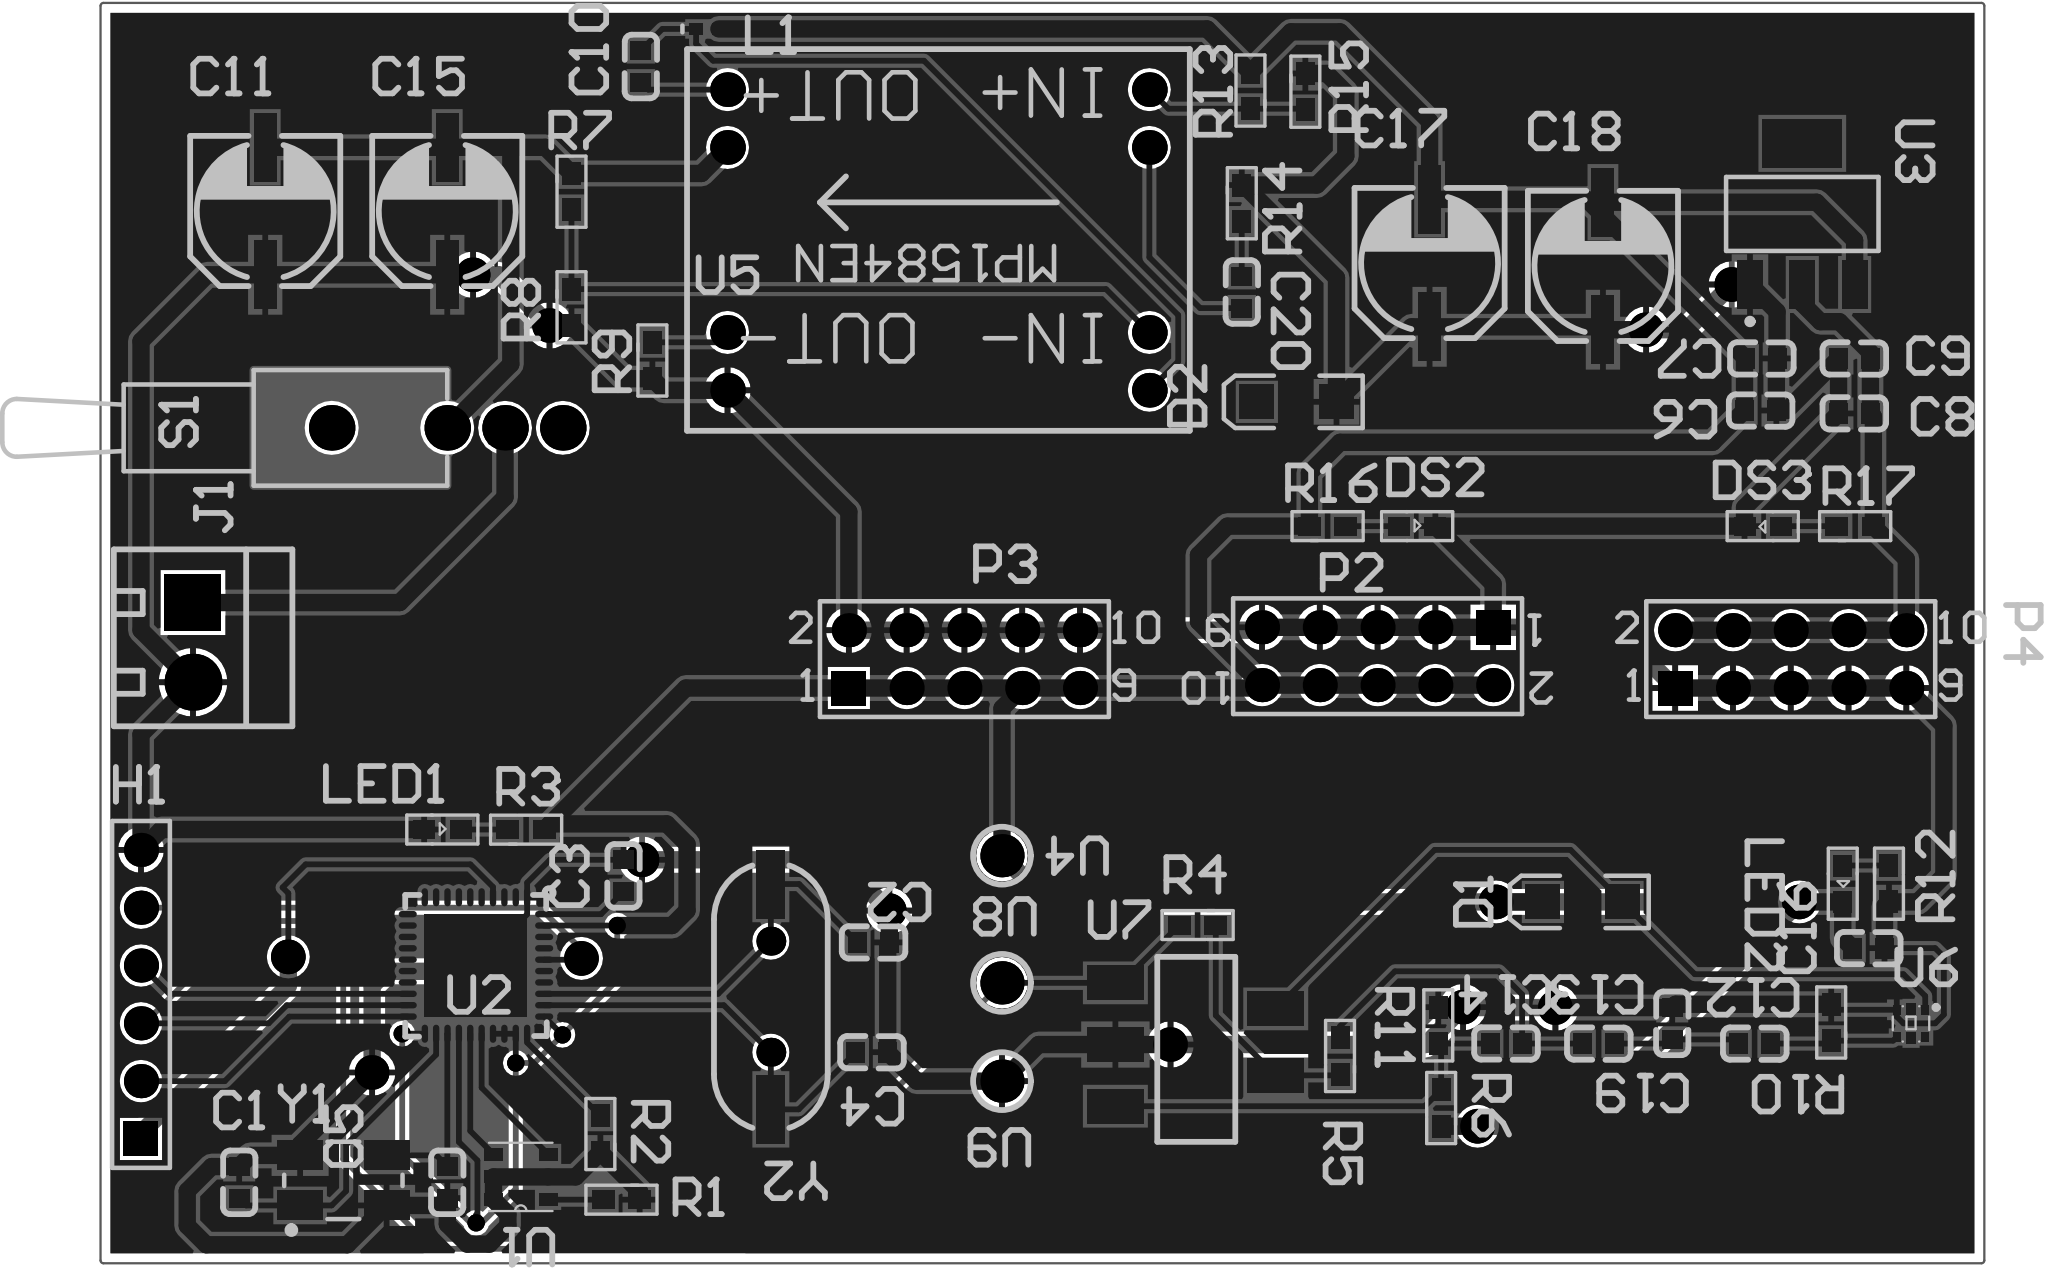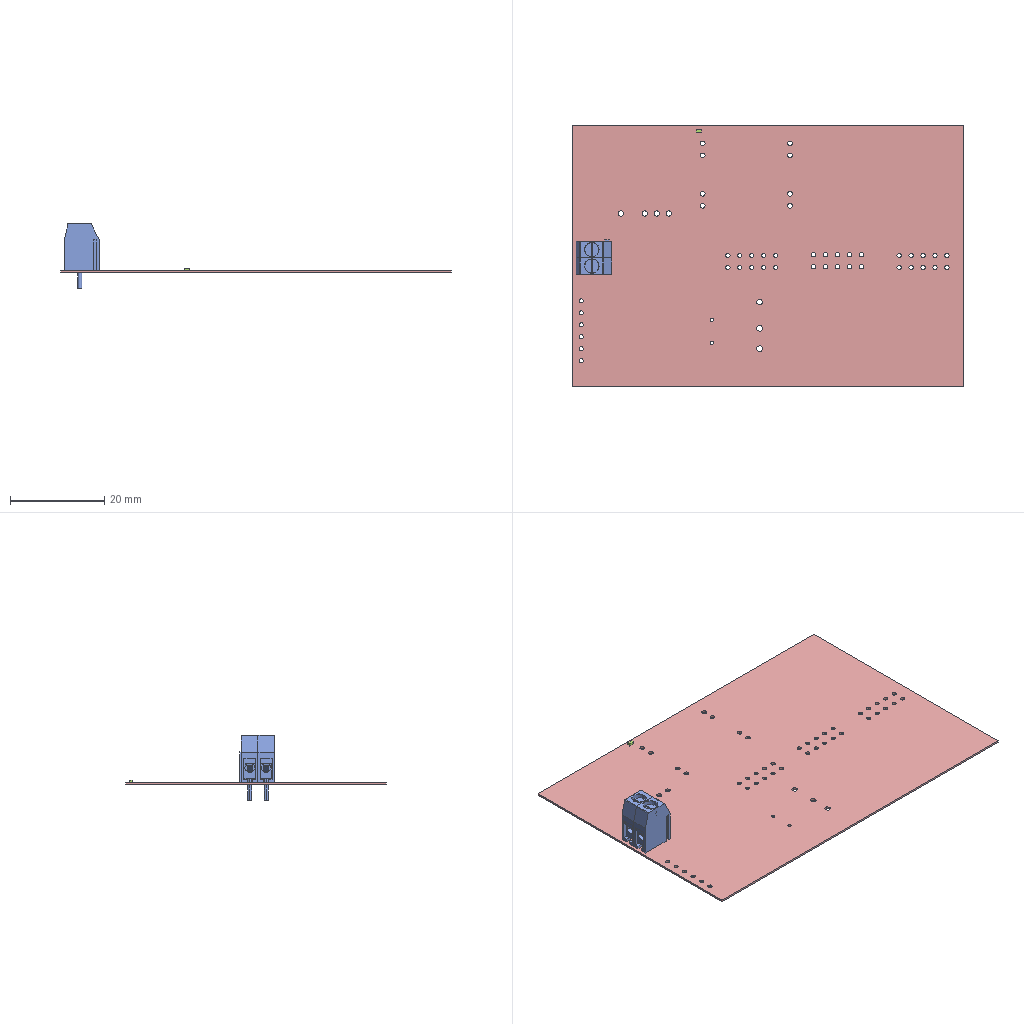Circuit board layout | Altium Designer | box 82.8 x 55.4 x 13.8 mm
Layer stack:
# Altium Designer layer stack of  (unit mm; dielectric type: 0 none, 1 core, 2 prepreg, 3 surface material)
index,name,kind,layer,copper_thickness_mm,dielectric_type,dielectric_thickness_mm,dielectric_material,dielectric_constant
0,Top Paste,other,,,,,,
1,Top Overlay,other,,,,,,
2,Top Solder,dielectric,,,3,0.0102,Solder Resist,3.5
3,Top Layer,copper,Top Layer,0.0356,,,,
4,Dielectric 1,dielectric,,,0,0.32,FR-4,4.8
5,Bottom Layer,copper,Bottom Layer,0.0356,,,,
6,Bottom Solder,dielectric,,,3,0.0102,Solder Resist,3.5
7,Bottom Overlay,other,,,,,,
8,Bottom Paste,other,,,,,,
# drill layer pairs: low layer,high layer
drill_pair,Top Layer,Bottom Layer
Part placement:
Designator,Comment,Layer,Footprint,Center-X(mm),Center-Y(mm),Rotation
C1,100nF,TopLayer,C0603,38.351,63.746,270
C2,100nF,TopLayer,C0603,66.229,74.295,180
C3,100nF,TopLayer,C0603,55.248,77.224,90
C4,100nF,TopLayer,C0603,66.159,69.472,180
C5,100nF,TopLayer,C0603,47.501,63.762,90
C6,100nF,TopLayer,C0603,105.221,97.663,180
C7,100nF,TopLayer,C0603,105.275,99.952,180
C8,100nF,TopLayer,C0603,109.355,97.533,0
C9,100nF,TopLayer,C0603,109.355,99.946,0
C10,100nF,TopLayer,C0603,56.01,112.784,90
C11,220UF/25V,TopLayer,贴片电容,39.497,106.426,360
C12,100nF,TopLayer,C0603,104.964,69.85,180
C13,100nF,TopLayer,C0603,98.109,69.85,180
C14,100nF,TopLayer,C0603,94.045,69.85,360
C15,10UF/50V,TopLayer,贴片电容,47.498,106.426,0
C16,100nF,TopLayer,C0603,109.974,74.044,180
C17,22UF/50V,TopLayer,贴片电容,90.678,104.14,0
C18,220UF/25V,TopLayer,贴片电容,98.298,104.013,0
C19,100nF,TopLayer,C0603,101.343,70.731,270
C20,100nF,TopLayer,C0603,82.42,102.862,270
D1,D_1N4007A,TopLayer,3.2X1.6X1.1,97.409,76.073,180
D2,Diode BAS16,TopLayer,3.2X1.6X1.1,84.836,98.044,180
DS2,LED2,TopLayer,my0603LED,90.132,92.583,360
DS3,LED2,TopLayer,my0603LED,105.321,92.583,180
H1,HDR-F_2.54_1x6P,TopLayer,HDR1X6,34.036,72.009,90
J1,KF350-2P,TopLayer,KF350-2P,36.322,87.475,270
L1,10UH,TopLayer,0402-A,58.936,114.427,0
LED1,LED_0603-R,TopLayer,my0603LED,47.282,79.254,360
LED2,LED_0603-R,TopLayer,my0603LED,108.839,76.873,270
P2,Header 5X2,TopLayer,HDR2X5,88.392,86.868,180
P3,Header 5X2,TopLayer,HDR2X5,70.231,86.741,360
P4,Header 5X2,TopLayer,HDR2X5,106.553,86.741,360
R1,10K,TopLayer,my0603,55.156,62.992,360
R2,10K,TopLayer,my0603,54.229,65.875,270
R3,10K,TopLayer,my0603,50.965,79.248,180
R4,10K,TopLayer,my0603,80.48,75.057,360
R5,10K,TopLayer,my0603,86.741,69.304,270
R6,10K,TopLayer,my0603,91.186,67.018,270
R7,10K,TopLayer,my0603,52.959,107.277,90
R8,10K,TopLayer,my0603,52.959,102.197,90
R9,10K,TopLayer,my0603,56.515,99.86,90
R10,10K,TopLayer,my0603,108.331,70.777,270
R11,10K,TopLayer,my0603,91.059,70.65,270
R12,10K,TopLayer,my0603,110.871,76.873,90
R13,10K,TopLayer,my0603,82.804,111.722,270
R14,10K,TopLayer,my0603,82.423,106.769,90
R15,10K,TopLayer,my0603,85.217,111.671,90
R16,10K,TopLayer,my0603,86.195,92.583,180
R17,10K,TopLayer,my0603,109.385,92.583,180
S1,SW-SPDT,TopLayer,TL36WW15050,47.498,96.901,180
U1,BL1,TopLayer,TSOP-6_-_duplicate,50.73,63.992,180
U2,CC2540,TopLayer,CC254X_QFN,48.76,73.279,270
U3,LM1117-3.3,TopLayer,LM1117-3.3,107.061,106.299,270
U4,RH-5000,TopLayer,TEST-TH_BD2.54-P1.4_RED,71.882,78.105,180
U5,MP1584EN,TopLayer,MP1548EN,69.089,105.156,180
U6,APDS,TopLayer,SENSORS-SMD_APDS-9008-020,111.839,70.739,360
U7,AMP,TopLayer,MCP6001,80.391,69.808,360
U8,RH-5000,TopLayer,TEST-TH_BD2.54-P1.4_RED,71.882,72.517,180
U9,RH-5000,TopLayer,TEST-TH_BD2.54-P1.4_RED,71.882,68.199,180
Y1,12MHz,TopLayer,OSC-SMD_4P-L5.0-W3.2-BL,42.931,63.838,360
Y2,8MHz,TopLayer,XTAL_US,61.722,71.909,270
Pad and via stacks:
# Altium Designer via and pad stacks of  (unit mm). Each distinct definition once, with the count of objects using it.
# via: kind,start_layer,end_layer,hole_mm,diameter_mm,mode(0 simple;1 top-mid-bottom;2 full stack),diameter_per_layer,count,example_net
# pad: kind,layer,hole_mm,hole_type(0 round;1 square;2 slot),plating,top_size,top_shape(1 round;2 rect;3 octagon;9 rounded rect),mid_size,bottom_size,mode,footprint,size_per_layer,count,example
pad,Top Layer,0,0,plated,1x0.8,2,1x0.8,1x0.8,0,my0603,,34,R16.2
pad,Top Layer,0,0,plated,0.965x0.8,2,0.965x0.8,0.965x0.8,0,my0603LED,,8,DS3.1
pad,Top Layer,0,0,plated,0.8x0.9,2,0.8x0.9,0.8x0.9,0,C0603,,32,C20.2
pad,Top Layer,0,0,plated,3x1,2,3x1,3x1,0,\u00CC\u00F9\u00C6\u00AC\u00B5\u00E7\u00C8\u00DD,,8,C17.1
pad,Top Layer,0,0,plated,1.5x1.5,2,1.5x1.5,1.5x1.5,0,3.2X1.6X1.1,,4,D2.2
pad,Top Layer,0,0,plated,0.35x0.4,2,0.35x0.4,0.35x0.4,0,SENSORS-SMD_APDS-9008-020,,4,U6.6
pad,Top Layer,0,0,plated,0.5x0.4,2,0.5x0.4,0.5x0.4,0,SENSORS-SMD_APDS-9008-020,,2,U6.5
pad,Top Layer,0,0,plated,2.5x1.524,2,2.5x1.524,2.5x1.524,0,MCP6001,,5,U7.5
pad,Top Layer,0,0,plated,0.5x0.6,2,0.5x0.6,0.5x0.6,0,0402-A,,2,L1.1
pad,Top Layer,0,0,plated,3x1.27,2,3x1.27,3x1.27,0,XTAL_US,,2,Y2.1
pad,Top Layer,0,0,plated,1.1x2.15,2,1.1x2.15,1.1x2.15,0,LM1117-3.3,,3,U3.1
pad,Top Layer,0,0,plated,3.5x2.15,2,3.5x2.15,3.5x2.15,0,LM1117-3.3,,1,U3.4
pad,Top Layer,0,0,plated,2x1.3,2,2x1.3,2x1.3,0,OSC-SMD_4P-L5.0-W3.2-BL,,4,Y1.3
pad,Top Layer,0,0,plated,0.28x0.8,1,0.28x0.8,0.28x0.8,0,CC254X_QFN,,40,U2.38
pad,Top Layer,0,0,plated,4.5x4.5,2,4.5x4.5,4.5x4.5,0,CC254X_QFN,,1,U2.41
pad,Top Layer,0,0,plated,0.8x0.55,2,0.8x0.55,0.8x0.55,0,TSOP-6 - duplicate,,6,U1.5
pad,Multi-Layer,0.9,0,plated,1.5x1.5,2,1.5x1.5,1.5x1.5,0,HDR2X5,,3,P2.1
pad,Multi-Layer,0.9,0,plated,1.5x1.5,1,1.5x1.5,1.5x1.5,0,HDR2X5,,27,P2.2
pad,Multi-Layer,1.2,0,plated,1.9x1.9,1,1.9x1.9,1.9x1.9,0,TEST-TH_BD2.54-P1.4_RED,,3,U9.1
pad,Multi-Layer,1,0,plated,1.524x1.524,1,1.524x1.524,1.524x1.524,0,MP1548EN,,8,U5.8
pad,Multi-Layer,1.1,0,plated,2x2,1,2x2,2x2,0,TL36WW15050,,4,S1.3
pad,Multi-Layer,1.5,0,plated,2.5x2.5,2,2.5x2.5,2.5x2.5,0,KF350-2P,,1,J1.1
pad,Multi-Layer,1.5,0,plated,2.5x2.5,1,2.5x2.5,2.5x2.5,0,KF350-2P,,1,J1.2
pad,Multi-Layer,0.7112,0,plated,1.27x1.27,1,1.27x1.27,1.27x1.27,0,XTAL_US,,2,Y2.1
pad,Multi-Layer,0.9,0,plated,1.5x1.5,1,1.5x1.5,1.5x1.5,0,HDR1X6,,5,H1.6
pad,Multi-Layer,0.9,0,plated,1.5x1.5,2,1.5x1.5,1.5x1.5,0,HDR1X6,,1,H1.1
via,Top Layer,Bottom Layer,0.762,1.524,0,,16,VCC
via,Top Layer,Bottom Layer,0.381,0.762,0,,5,VCC
Copper pours:
name,layer,net,type(0 solid;1 hatched;2 none)
Top Layer-No Net,Top Layer,GND,0
Top Layer-No Net,Bottom Layer,GND,0
Design rules, without the lines most boards share:
# Altium Designer design rules of  (exported by Altium Designer, unit mm)
# columns: name | kind | enabled | priority | scope1 | scope2 | descriptor | typed fields (field=value)
SilkToSilkClearance | 55 | enabled | 1 | All | All | Silk to Silk (Clearance=0mil) (All),(All) |
SilkToSolderMaskClearance | 54 | enabled | 1 | IsPad | All | Silk To Solder Mask (Clearance=0mil) (IsPad),(All) |
MinimumSolderMaskSliver | 53 | enabled | 1 | All | All | Minimum Solder Mask Sliver (Gap=0mil) (All),(All) |
HoleToHoleClearance | 52 | enabled | 1 | All | All | Hole To Hole Clearance (Gap=10mil) (All),(All) | gap=0.254
DiffPairsRouting | 51 | enabled | 1 | All | All | Differential Pairs Uncoupled Length using the Gap Constraints (Min=10mil) (Max=10mil) (Prefered=10mil)  and Width Constraints (Min=15mil) (Max=15mil) (Prefered=15mil) (All) |
SolderMaskExpansion | 13 | enabled | 1 | All | All | Solder Mask Expansion (Expansion =4mil) (All) | expansion=0.1016
PasteMaskExpansion | 14 | enabled | 1 | All | All | Paste Mask Expansion (Expansion =0mil) (All) | expansion=0
RoutingVias | 11 | enabled | 1 | All | All | Routing Via (MinHoleWidth=28mil) (MaxHoleWidth=28mil) (PreferredHoleWidth=28mil) (MinWidth=50mil) (MaxWidth=50mil) (PreferedWidth=50mil) (All) | via_min_hole=0.7112 via_max_hole=0.7112 via_preferred_diameter=1.27 via_preferred_hole=0.7112
Width | 2 | enabled | 1 | All | All | Width Constraint (Min=10mil) (Max=30mil) (Preferred=10mil) (All) |
PolygonConnect | 20 | enabled | 1 | All | All | Polygon Connect Rule(Relief Connect )(Conductor Width=10mil) (Relief Angle=90 Angle) (Entries=4) (Air Gap Width=10mil) (All),(All) | connect_style(0=relief,1=direct,2=none)=0 relief_conductor_width=0.254 relief_entries=4
PlaneConnect | 6 | enabled | 1 | All | All | Power Plane Connect Rule(Relief Connect )(Expansion=20mil) (Conductor Width=10mil) (Air Gap=10mil) (Entries=4) (All) | relief_conductor_width=0.254 relief_entries=4 relief_expansion=0.508
Clearance | 0 | enabled | 1 | All | All | Clearance Constraint (Gap=7mil) (All),(All) | gap=0.1778
Classes set for this board:
# Altium Designer classes of  (member kind: 0 net, 1 component, 2 from-to, 3 pad, 4 layer, 5 differential pair, 6 design channel, 7 polygon, 8 structure, 9 xSignal)
# columns: class name | member kind | superclass | members
3_P1 | 1 | no | C1; C2; C3; C4; C5; C6; C7; C8; C9; C10; C11; C12; C13; C14; C15; C16; C17; C18; C19; C20; D1; D2; DS2; DS3; H1; J1; L1; LED1; LED2; P2; P3; P4; R1; R2; R3; R4; R5; R6; R7; R8; R9; R10; R11; R12; R13; R14; R15; R16; R17; S1; U1; U2; U3; U4; U5; U6; U7; U8; U9; Y1; Y2;